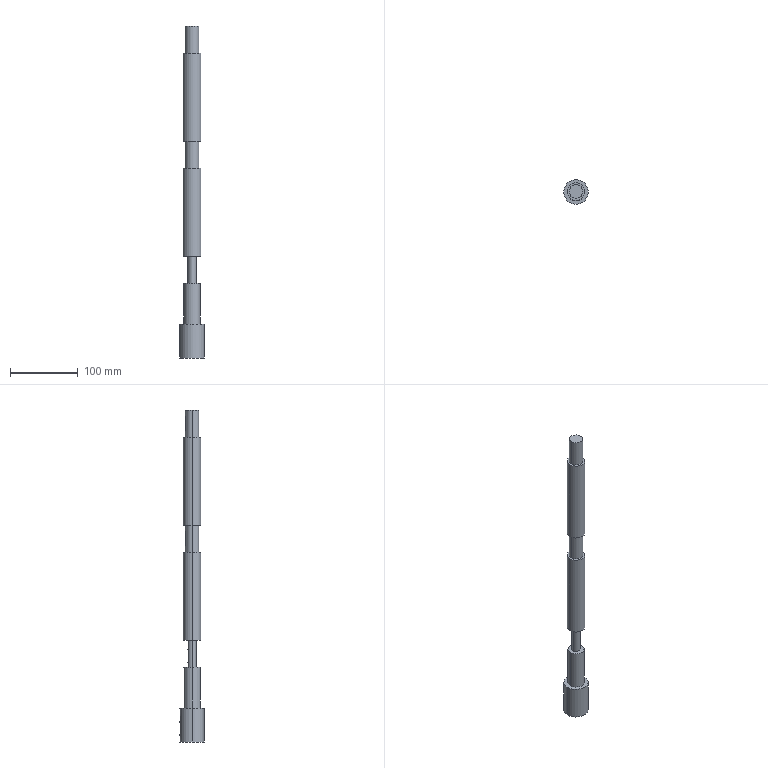Part | SolidWorks | features ICE 6, Extrusion 1, Revolution 1 | 1 solid | 46 faces | box 36 x 36 x 490 mm | volume 244254 mm3 | cylinder 26 | plane 20 | commonest cylinder face diameters 5 x6 20 x4 26 x4 2.8 x3 10 x3 12 x2